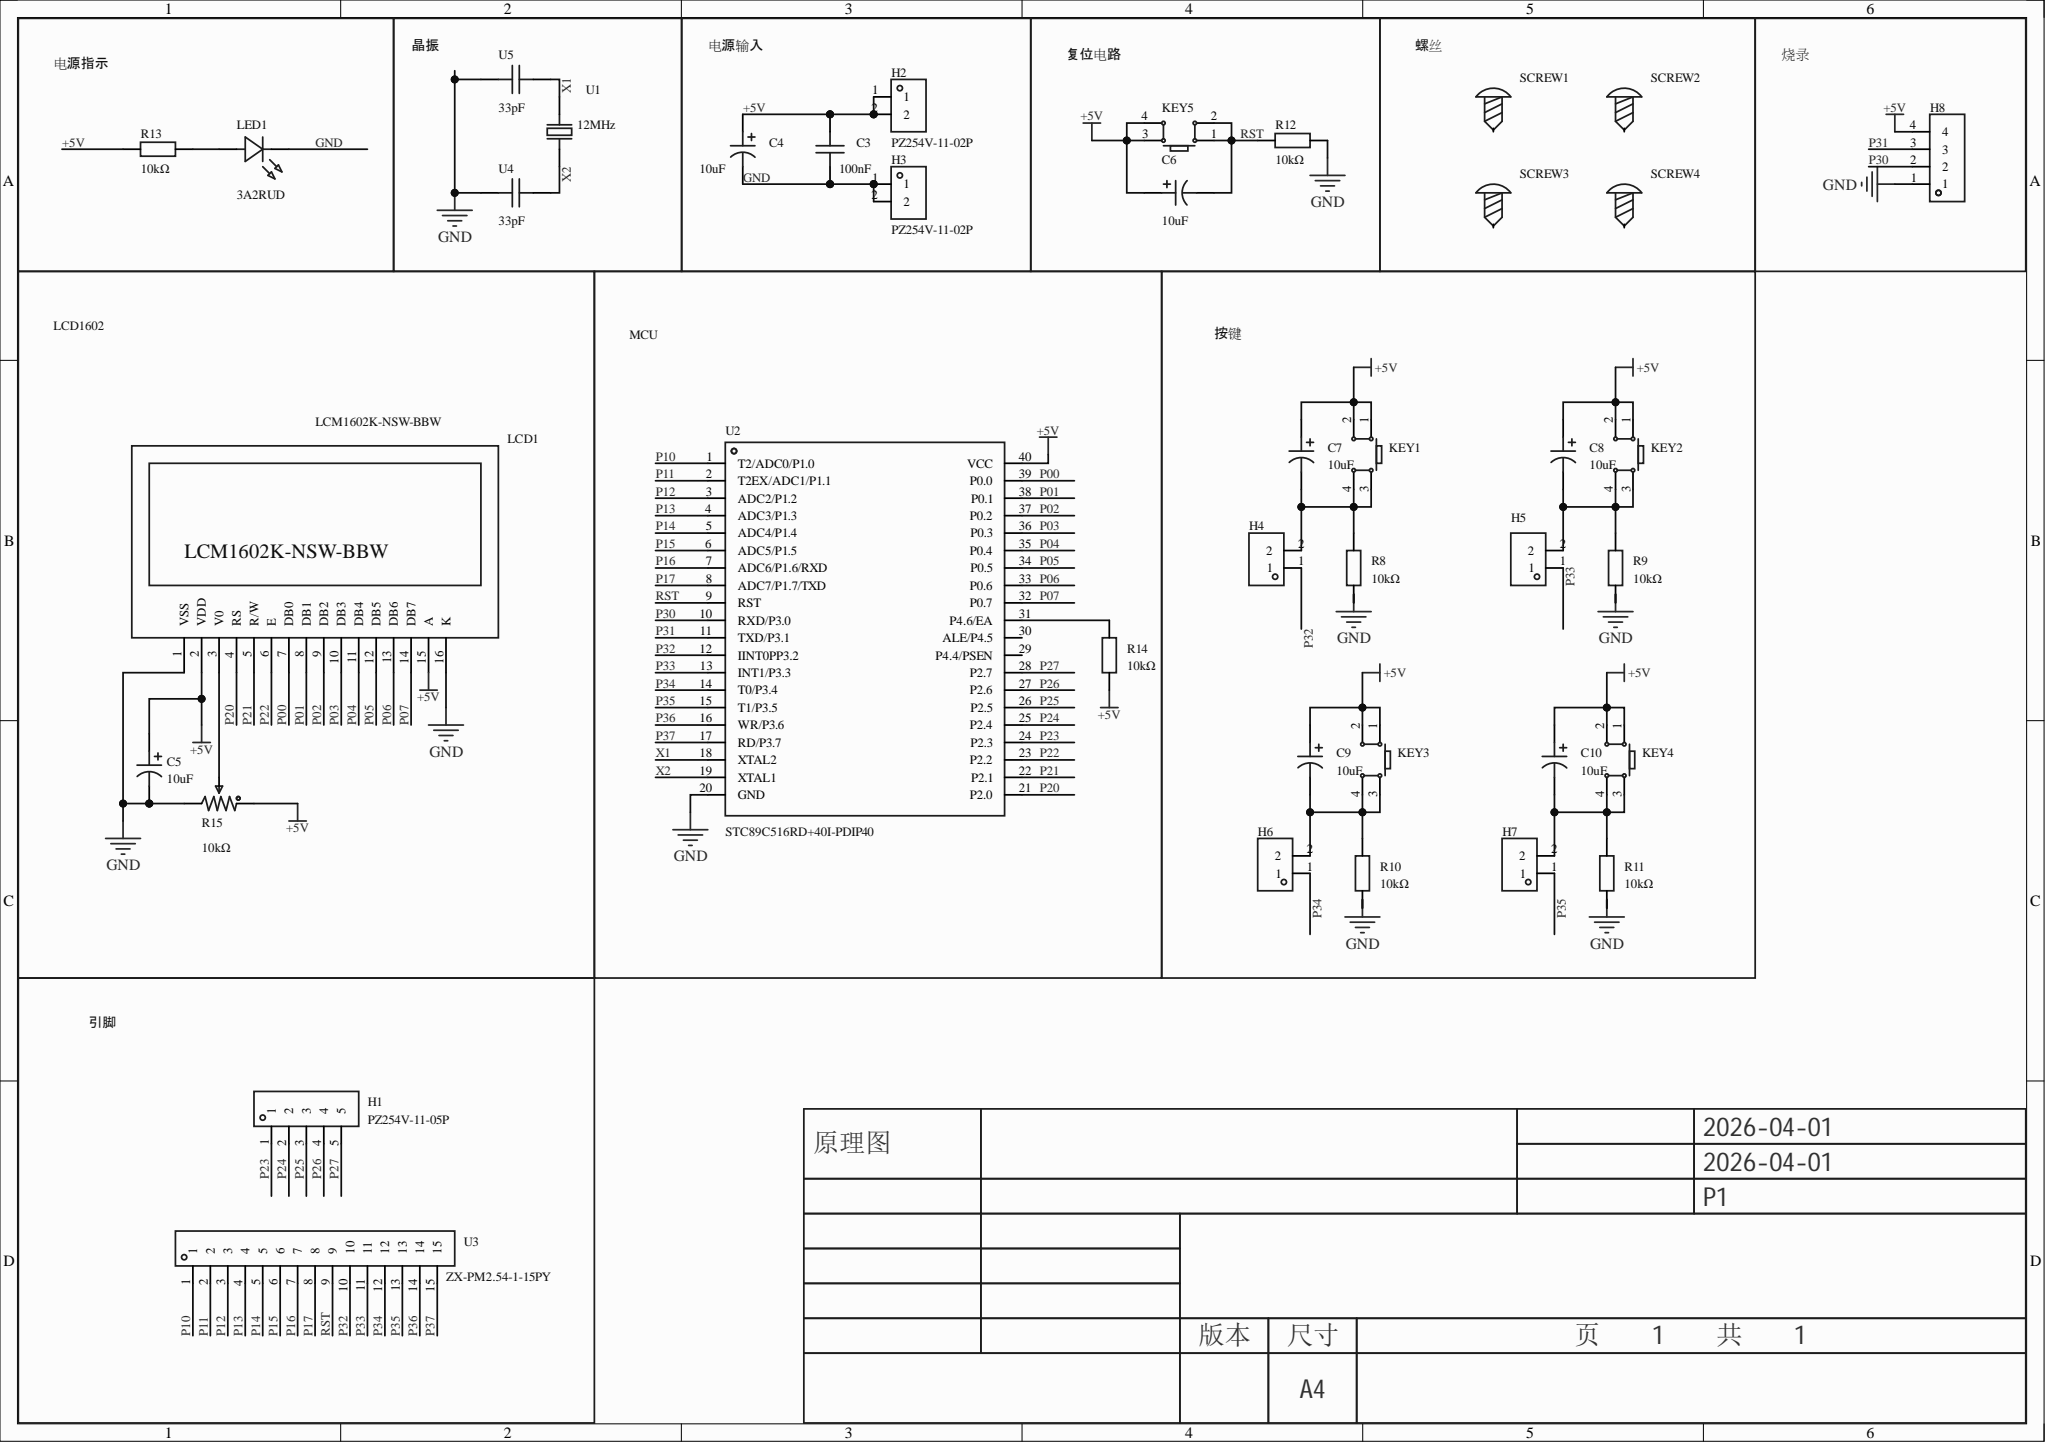Circuit board | Altium Designer | 40 parts | 44 nets
Bill of materials:
Comment,Description,Designator,Footprint,LibRef,Quantity
"100nF","","C3","CAP-TH_L5.0-W2.5-P5.00-D1.0","CC1H104MC1FD3F6C10MF","1"
"10uF","","C4, C5, C6, C7, C8, C9, C10","CAP-TH_BD5.0-P2.00-D0.5-FD-A","ERG50V10M5X11","7"
"PZ254V-11-05P","","H1","HDR-TH_5P-P2.54-V-M","PZ254V-11-05P","1"
"PZ254V-11-02P","","H2, H3, H4, H5, H6, H7","HDR-TH_2P-P2.54-V-M","PZ254V-11-02P","6"
"","","H8","HDR-TH_4P-P2.54-V-F","HDR-F_2.54_1x4P","1"
"","","KEY1, KEY2, KEY3, KEY4, KEY5","SW-TH_4P-L6.0-W6.0-P4.50-LS6.5","Key_TH_6x6x6","5"
"LCM1602K-NSW-BBW","","LCD1","MODULE-TH_LCM1602K","LCM1602K-NSW-BBW","1"
"3A2RUD","","LED1","LED-TH_BD3.5-P2.28_3A2RUC","3A2RUD","1"
"10kΩ","","R8, R9, R10, R11, R12, R13, R14","RES-TH_BD2.3-L6.5-P10.50-D0.5","MF1/4W-10KΩ±1% T","7"
"10kΩ","","R15","RES-ADJ-TH_3P-L10.0-W10.0-P2.50-L","3296W-1-103","1"
"","","SCREW1, SCREW2, SCREW3, SCREW4","M2螺丝","M2螺丝","4"
"12MHz","","U1","HC-49S_L11.0-W4.7-P4.88","YG12MLBBE2X","1"
"STC89C516RD+40I-PDIP40","","U2","DIP-40_L52.3-W13.9-P2.54-LS15.2-BL","STC89C516RD+40I-PDIP40","1"
"ZX-PM2.54-1-15PY","","U3","HDR-TH_15P-P2.54-V-F","ZX-PM2.54-1-15PY","1"
"33pF","","U4, U5","CAP-TH_L5.0-W2.5-P5.08-D0.7","CC1H330JC74DCH4B10MN","2"
Netlist (Protel format):
[
C3
CAP-TH_L5.0-W2.5-P5.00-D1.0
100nF



]
[
C4
CAP-TH_BD5.0-P2.00-D0.5-FD-A
10uF



]
[
C5
CAP-TH_BD5.0-P2.00-D0.5-FD-A
10uF



]
[
C6
CAP-TH_BD5.0-P2.00-D0.5-FD-A
10uF



]
[
C7
CAP-TH_BD5.0-P2.00-D0.5-FD-A
10uF



]
[
C8
CAP-TH_BD5.0-P2.00-D0.5-FD-A
10uF



]
[
C9
CAP-TH_BD5.0-P2.00-D0.5-FD-A
10uF



]
[
C10
CAP-TH_BD5.0-P2.00-D0.5-FD-A
10uF



]
[
H1
HDR-TH_5P-P2.54-V-M
PZ254V-11-05P



]
[
H2
HDR-TH_2P-P2.54-V-M
PZ254V-11-02P



]
[
H3
HDR-TH_2P-P2.54-V-M
PZ254V-11-02P



]
[
H4
HDR-TH_2P-P2.54-V-M
PZ254V-11-02P



]
[
H5
HDR-TH_2P-P2.54-V-M
PZ254V-11-02P



]
[
H6
HDR-TH_2P-P2.54-V-M
PZ254V-11-02P



]
[
H7
HDR-TH_2P-P2.54-V-M
PZ254V-11-02P



]
[
H8
HDR-TH_4P-P2.54-V-F




]
[
KEY1
SW-TH_4P-L6.0-W6.0-P4.50-LS6.5




]
[
KEY2
SW-TH_4P-L6.0-W6.0-P4.50-LS6.5




]
[
KEY3
SW-TH_4P-L6.0-W6.0-P4.50-LS6.5




]
[
KEY4
SW-TH_4P-L6.0-W6.0-P4.50-LS6.5




]
[
KEY5
SW-TH_4P-L6.0-W6.0-P4.50-LS6.5




]
[
LCD1
MODULE-TH_LCM1602K
LCM1602K-NSW-BBW



]
[
LED1
LED-TH_BD3.5-P2.28_3A2RUC
3A2RUD



]
[
R8
RES-TH_BD2.3-L6.5-P10.50-D0.5
10kΩ



]
[
R9
RES-TH_BD2.3-L6.5-P10.50-D0.5
10kΩ



]
[
R10
RES-TH_BD2.3-L6.5-P10.50-D0.5
10kΩ



]
[
R11
RES-TH_BD2.3-L6.5-P10.50-D0.5
10kΩ



]
[
R12
RES-TH_BD2.3-L6.5-P10.50-D0.5
10kΩ



]
[
R13
RES-TH_BD2.3-L6.5-P10.50-D0.5
10kΩ



]
[
R14
RES-TH_BD2.3-L6.5-P10.50-D0.5
10kΩ



]
[
R15
RES-ADJ-TH_3P-L10.0-W10.0-P2.50-L
10kΩ



]
[
SCREW1
M2螺丝




]
[
SCREW2
M2螺丝




]
[
SCREW3
M2螺丝




]
[
SCREW4
M2螺丝




]
[
U1
HC-49S_L11.0-W4.7-P4.88
12MHz



]
[
U2
DIP-40_L52.3-W13.9-P2.54-LS15.2-BL
STC89C516RD+40I-PDIP40



]
[
U3
HDR-TH_15P-P2.54-V-F
ZX-PM2.54-1-15PY



]
[
U4
CAP-TH_L5.0-W2.5-P5.08-D0.7
33pF



]
[
U5
CAP-TH_L5.0-W2.5-P5.08-D0.7
33pF



]
(
X2
U1-1
U2-19
U4-2
)
(
X1
U1-2
U2-18
U5-2
)
(
RST
C6-2
KEY5-1
KEY5-2
R12-2
U2-9
U3-9
)
(
P37
U2-17
U3-15
)
(
P36
U2-16
U3-14
)
(
P35
H7-1
U2-15
U3-13
)
(
P34
H6-1
U2-14
U3-12
)
(
P33
H5-1
U2-13
U3-11
)
(
P32
H4-1
U2-12
U3-10
)
(
P31
H8-3
U2-11
)
(
P30
H8-2
U2-10
)
(
P27
H1-5
U2-28
)
(
P26
H1-4
U2-27
)
(
P25
H1-3
U2-26
)
(
P24
H1-2
U2-25
)
(
P23
H1-1
U2-24
)
(
P22
LCD1-6
U2-23
)
(
P21
LCD1-5
U2-22
)
(
P20
LCD1-4
U2-21
)
(
P17
U2-8
U3-8
)
(
P16
U2-7
U3-7
)
(
P15
U2-6
U3-6
)
(
P14
U2-5
U3-5
)
(
P13
U2-4
U3-4
)
(
P12
U2-3
U3-3
)
(
P11
U2-2
U3-2
)
(
P10
U2-1
U3-1
)
(
P07
LCD1-14
U2-32
)
(
P06
LCD1-13
U2-33
)
(
P05
LCD1-12
U2-34
)
(
P04
LCD1-11
U2-35
)
(
P03
LCD1-10
U2-36
)
(
P02
LCD1-9
U2-37
)
(
P01
LCD1-8
U2-38
)
(
P00
LCD1-7
U2-39
)
(
NetR14_2
R14-2
U2-31
)
(
NetLED1_2
LED1-2
R13-1
)
(
NetLCD1_3
LCD1-3
R15-2
)
(
NetC10_2
C10-2
H7-2
KEY4-3
KEY4-4
R11-2
)
(
NetC9_2
C9-2
H6-2
KEY3-3
KEY3-4
R10-2
)
(
NetC8_2
C8-2
H5-2
KEY2-3
KEY2-4
R9-2
)
(
NetC7_2
C7-2
H4-2
KEY1-3
KEY1-4
R8-2
)
(
GND
C3-1
C4-2
C5-2
H3-1
H3-2
H8-1
LCD1-1
LCD1-16
LED1-1
R8-1
R9-1
R10-1
R11-1
R12-1
R15-3
U2-20
U4-1
U5-1
)
(
+5V
C3-2
C4-1
C5-1
C6-1
C7-1
C8-1
C9-1
C10-1
H2-1
H2-2
H8-4
KEY1-1
KEY1-2
KEY2-1
KEY2-2
KEY3-1
KEY3-2
KEY4-1
KEY4-2
KEY5-3
KEY5-4
LCD1-2
LCD1-15
R13-2
R14-1
R15-1
U2-40
)